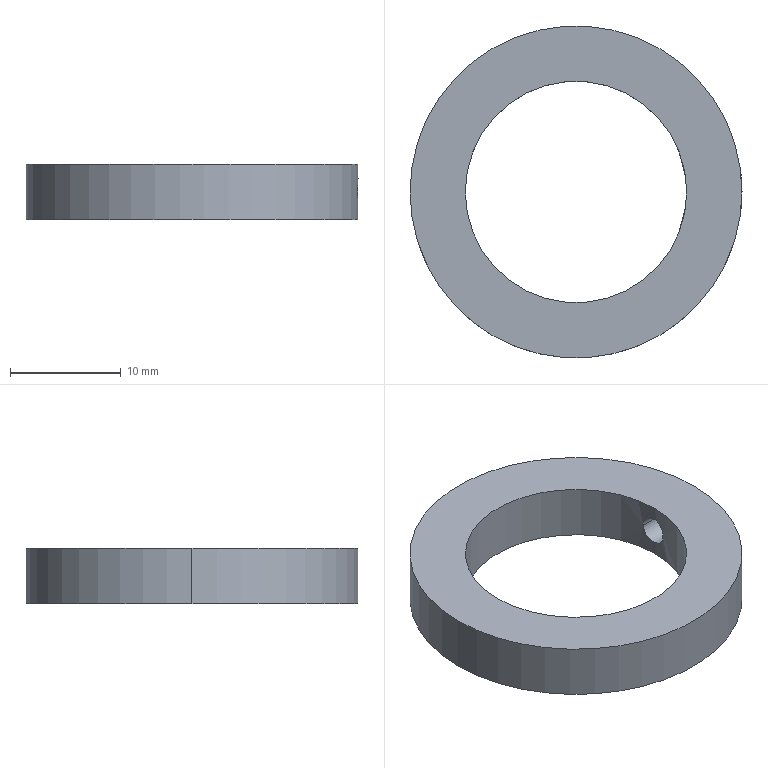Part | SolidWorks | features 3DProfileFeature 1, Extrusion 1, HoleWzd 1 | 1 solid | 8 faces | box 30 x 30 x 5 mm | volume 1939 mm3 | cylinder 6 | plane 2 | commonest cylinder face diameters 2.5 x2 20 x2 30 x2
STEP:
#1=CARTESIAN_POINT('',(10.,0.,1.252));
#2=VERTEX_POINT('',#1);
#3=CARTESIAN_POINT('',(9.93,-1.183,2.5));
#4=VERTEX_POINT('',#3);
#5=CARTESIAN_POINT('',(10.,0.,1.252));
#6=CARTESIAN_POINT('',(10.,-0.1581,1.26));
#7=CARTESIAN_POINT('',(9.996,-0.3132,1.299));
#8=CARTESIAN_POINT('',(9.983,-0.602,1.433));
#9=CARTESIAN_POINT('',(9.974,-0.7312,1.525));
#10=CARTESIAN_POINT('',(9.955,-0.9493,1.756));
#11=CARTESIAN_POINT('',(9.946,-1.035,1.891));
#12=CARTESIAN_POINT('',(9.934,-1.152,2.184));
#13=CARTESIAN_POINT('',(9.93,-1.183,2.342));
#14=CARTESIAN_POINT('',(9.93,-1.183,2.5));
#15=B_SPLINE_CURVE_WITH_KNOTS('',3,(#5,#6,#7,#8,#9,#10,#11,#12,#13,#14),.UNSPECIFIED.,.F.,.F.,(4,2,2,2,4),(0.002024,0.002496,0.002968,0.00344,0.003912),.UNSPECIFIED.);
#16=EDGE_CURVE('',#2,#4,#15,.T.);
#17=ORIENTED_EDGE('',*,*,#16,.T.);
#18=CARTESIAN_POINT('',(14.956,-1.149,2.5));
#19=VERTEX_POINT('',#18);
#20=CARTESIAN_POINT('',(15.008,-1.148,2.5));
#21=DIRECTION('',(1.,0.00677,0.));
#22=VECTOR('',#21,1000.);
#23=LINE('',#20,#22);
#24=EDGE_CURVE('',#4,#19,#23,.T.);
#25=ORIENTED_EDGE('',*,*,#24,.T.);
#26=CARTESIAN_POINT('',(15.,0.,1.254));
#27=VERTEX_POINT('',#26);
#28=CARTESIAN_POINT('',(15.,0.,1.254));
#29=CARTESIAN_POINT('',(15.,-0.3107,1.279));
#30=CARTESIAN_POINT('',(14.989,-0.6069,1.424));
#31=CARTESIAN_POINT('',(14.972,-0.9234,1.767));
#32=CARTESIAN_POINT('',(14.966,-1.007,1.901));
#33=CARTESIAN_POINT('',(14.958,-1.12,2.19));
#34=CARTESIAN_POINT('',(14.956,-1.149,2.345));
#35=CARTESIAN_POINT('',(14.956,-1.149,2.5));
#36=B_SPLINE_CURVE_WITH_KNOTS('',3,(#28,#29,#30,#31,#32,#33,#34,#35),.UNSPECIFIED.,.F.,.F.,(4,2,2,4),(0.002057,0.002983,0.003446,0.00391),.UNSPECIFIED.);
#37=EDGE_CURVE('',#27,#19,#36,.T.);
#38=ORIENTED_EDGE('',*,*,#37,.F.);
#39=CARTESIAN_POINT('',(14.939,1.351,2.5));
#40=VERTEX_POINT('',#39);
#41=CARTESIAN_POINT('',(14.939,1.351,2.5));
#42=CARTESIAN_POINT('',(14.939,1.351,2.413));
#43=CARTESIAN_POINT('',(14.94,1.342,2.328));
#44=CARTESIAN_POINT('',(14.943,1.307,2.16));
#45=CARTESIAN_POINT('',(14.945,1.28,2.076));
#46=CARTESIAN_POINT('',(14.954,1.177,1.84));
#47=CARTESIAN_POINT('',(14.962,1.074,1.697));
#48=CARTESIAN_POINT('',(14.978,0.8225,1.465));
#49=CARTESIAN_POINT('',(14.986,0.671,1.374));
#50=CARTESIAN_POINT('',(14.994,0.4277,1.29));
#51=CARTESIAN_POINT('',(14.996,0.3423,1.27));
#52=CARTESIAN_POINT('',(14.999,0.1719,1.249));
#53=CARTESIAN_POINT('',(15.,0.0862,1.247));
#54=CARTESIAN_POINT('',(15.,0.,1.254));
#55=B_SPLINE_CURVE_WITH_KNOTS('',3,(#41,#42,#43,#44,#45,#46,#47,#48,#49,#50,#51,#52,#53,#54),.UNSPECIFIED.,.F.,.F.,(4,2,2,2,2,2,4),(0.,0.0002571,0.0005141,0.001028,0.001542,0.001799,0.002057),.UNSPECIFIED.);
#56=EDGE_CURVE('',#40,#27,#55,.T.);
#57=ORIENTED_EDGE('',*,*,#56,.F.);
#58=CARTESIAN_POINT('',(9.913,1.317,2.5));
#59=VERTEX_POINT('',#58);
#60=CARTESIAN_POINT('',(14.991,1.352,2.5));
#61=DIRECTION('',(1.,0.00677,0.));
#62=VECTOR('',#61,1000.);
#63=LINE('',#60,#62);
#64=EDGE_CURVE('',#59,#40,#63,.T.);
#65=ORIENTED_EDGE('',*,*,#64,.F.);
#66=CARTESIAN_POINT('',(9.913,1.317,2.5));
#67=CARTESIAN_POINT('',(9.913,1.317,2.414));
#68=CARTESIAN_POINT('',(9.914,1.308,2.33));
#69=CARTESIAN_POINT('',(9.918,1.274,2.165));
#70=CARTESIAN_POINT('',(9.922,1.249,2.083));
#71=CARTESIAN_POINT('',(9.934,1.148,1.85));
#72=CARTESIAN_POINT('',(9.946,1.049,1.708));
#73=CARTESIAN_POINT('',(9.968,0.8046,1.476));
#74=CARTESIAN_POINT('',(9.98,0.6572,1.385));
#75=CARTESIAN_POINT('',(9.991,0.4198,1.298));
#76=CARTESIAN_POINT('',(9.995,0.3364,1.276));
#77=CARTESIAN_POINT('',(9.999,0.1689,1.251));
#78=CARTESIAN_POINT('',(10.,0.08472,1.247));
#79=CARTESIAN_POINT('',(10.,0.,1.252));
#80=B_SPLINE_CURVE_WITH_KNOTS('',3,(#66,#67,#68,#69,#70,#71,#72,#73,#74,#75,#76,#77,#78,#79),.UNSPECIFIED.,.F.,.F.,(4,2,2,2,2,2,4),(0.,0.000253,0.000506,0.001012,0.001518,0.001771,0.002024),.UNSPECIFIED.);
#81=EDGE_CURVE('',#59,#2,#80,.T.);
#82=ORIENTED_EDGE('',*,*,#81,.T.);
#83=EDGE_LOOP('',(#17,#25,#38,#57,#65,#82));
#84=FACE_OUTER_BOUND('',#83,.T.);
#85=CARTESIAN_POINT('',(15.,0.1016,2.5));
#86=DIRECTION('',(1.,0.00677,0.));
#87=DIRECTION('',(-0.00677,1.,0.));
#88=AXIS2_PLACEMENT_3D('',#85,#86,#87);
#89=CYLINDRICAL_SURFACE('',#88,1.25);
#90=ADVANCED_FACE('',(#84),#89,.F.);
#91=CARTESIAN_POINT('',(-10.,0.,5.));
#92=VERTEX_POINT('',#91);
#93=CARTESIAN_POINT('',(10.,0.,5.));
#94=VERTEX_POINT('',#93);
#95=CARTESIAN_POINT('',(0.,0.,5.));
#96=DIRECTION('',(0.,0.,1.));
#97=DIRECTION('',(1.,0.,0.));
#98=AXIS2_PLACEMENT_3D('',#95,#96,#97);
#99=CIRCLE('',#98,10.);
#100=EDGE_CURVE('',#92,#94,#99,.T.);
#101=ORIENTED_EDGE('',*,*,#100,.T.);
#102=CARTESIAN_POINT('',(10.,0.,3.748));
#103=VERTEX_POINT('',#102);
#104=CARTESIAN_POINT('',(10.,0.,5.));
#105=DIRECTION('',(0.,0.,-1.));
#106=VECTOR('',#105,1000.);
#107=LINE('',#104,#106);
#108=EDGE_CURVE('',#94,#103,#107,.T.);
#109=ORIENTED_EDGE('',*,*,#108,.T.);
#110=CARTESIAN_POINT('',(9.93,-1.183,2.5));
#111=CARTESIAN_POINT('',(9.93,-1.183,2.658));
#112=CARTESIAN_POINT('',(9.934,-1.152,2.817));
#113=CARTESIAN_POINT('',(9.946,-1.036,3.109));
#114=CARTESIAN_POINT('',(9.956,-0.9483,3.245));
#115=CARTESIAN_POINT('',(9.974,-0.7319,3.474));
#116=CARTESIAN_POINT('',(9.983,-0.6007,3.568));
#117=CARTESIAN_POINT('',(9.996,-0.3145,3.701));
#118=CARTESIAN_POINT('',(10.,-0.1583,3.74));
#119=CARTESIAN_POINT('',(10.,0.,3.748));
#120=B_SPLINE_CURVE_WITH_KNOTS('',3,(#110,#111,#112,#113,#114,#115,#116,#117,#118,#119),.UNSPECIFIED.,.F.,.F.,(4,2,2,2,4),(0.003912,0.004384,0.004857,0.005329,0.005801),.UNSPECIFIED.);
#121=EDGE_CURVE('',#4,#103,#120,.T.);
#122=ORIENTED_EDGE('',*,*,#121,.F.);
#123=ORIENTED_EDGE('',*,*,#16,.F.);
#124=CARTESIAN_POINT('',(10.,0.,0.));
#125=VERTEX_POINT('',#124);
#126=CARTESIAN_POINT('',(10.,0.,5.));
#127=DIRECTION('',(0.,0.,-1.));
#128=VECTOR('',#127,1000.);
#129=LINE('',#126,#128);
#130=EDGE_CURVE('',#2,#125,#129,.T.);
#131=ORIENTED_EDGE('',*,*,#130,.T.);
#132=CARTESIAN_POINT('',(-10.,0.,0.));
#133=VERTEX_POINT('',#132);
#134=CARTESIAN_POINT('',(0.,0.,0.));
#135=DIRECTION('',(0.,0.,1.));
#136=DIRECTION('',(1.,0.,0.));
#137=AXIS2_PLACEMENT_3D('',#134,#135,#136);
#138=CIRCLE('',#137,10.);
#139=EDGE_CURVE('',#133,#125,#138,.T.);
#140=ORIENTED_EDGE('',*,*,#139,.F.);
#141=CARTESIAN_POINT('',(-10.,0.,5.));
#142=DIRECTION('',(0.,0.,-1.));
#143=VECTOR('',#142,1000.);
#144=LINE('',#141,#143);
#145=EDGE_CURVE('',#92,#133,#144,.T.);
#146=ORIENTED_EDGE('',*,*,#145,.F.);
#147=EDGE_LOOP('',(#101,#109,#122,#123,#131,#140,#146));
#148=FACE_OUTER_BOUND('',#147,.T.);
#149=CARTESIAN_POINT('',(0.,0.,5.));
#150=DIRECTION('',(0.,0.,-1.));
#151=DIRECTION('',(-1.,0.,0.));
#152=AXIS2_PLACEMENT_3D('',#149,#150,#151);
#153=CYLINDRICAL_SURFACE('',#152,10.);
#154=ADVANCED_FACE('',(#148),#153,.F.);
#155=CARTESIAN_POINT('',(15.,0.,5.));
#156=VERTEX_POINT('',#155);
#157=CARTESIAN_POINT('',(-15.,0.,5.));
#158=VERTEX_POINT('',#157);
#159=CARTESIAN_POINT('',(0.,0.,5.));
#160=DIRECTION('',(0.,0.,1.));
#161=DIRECTION('',(1.,0.,0.));
#162=AXIS2_PLACEMENT_3D('',#159,#160,#161);
#163=CIRCLE('',#162,15.);
#164=EDGE_CURVE('',#156,#158,#163,.T.);
#165=ORIENTED_EDGE('',*,*,#164,.F.);
#166=CARTESIAN_POINT('',(15.,0.,3.746));
#167=VERTEX_POINT('',#166);
#168=CARTESIAN_POINT('',(15.,0.,5.));
#169=DIRECTION('',(0.,0.,-1.));
#170=VECTOR('',#169,1000.);
#171=LINE('',#168,#170);
#172=EDGE_CURVE('',#156,#167,#171,.T.);
#173=ORIENTED_EDGE('',*,*,#172,.T.);
#174=CARTESIAN_POINT('',(15.,0.,3.746));
#175=CARTESIAN_POINT('',(15.,0.0856,3.753));
#176=CARTESIAN_POINT('',(14.999,0.1731,3.751));
#177=CARTESIAN_POINT('',(14.996,0.3431,3.729));
#178=CARTESIAN_POINT('',(14.994,0.4266,3.71));
#179=CARTESIAN_POINT('',(14.986,0.6724,3.625));
#180=CARTESIAN_POINT('',(14.978,0.8221,3.536));
#181=CARTESIAN_POINT('',(14.962,1.075,3.303));
#182=CARTESIAN_POINT('',(14.954,1.177,3.159));
#183=CARTESIAN_POINT('',(14.942,1.315,2.846));
#184=CARTESIAN_POINT('',(14.939,1.351,2.674));
#185=CARTESIAN_POINT('',(14.939,1.351,2.5));
#186=B_SPLINE_CURVE_WITH_KNOTS('',3,(#174,#175,#176,#177,#178,#179,#180,#181,#182,#183,#184,#185),.UNSPECIFIED.,.F.,.F.,(4,2,2,2,2,4),(0.005764,0.006021,0.006278,0.006791,0.007305,0.007819),.UNSPECIFIED.);
#187=EDGE_CURVE('',#167,#40,#186,.T.);
#188=ORIENTED_EDGE('',*,*,#187,.T.);
#189=ORIENTED_EDGE('',*,*,#56,.T.);
#190=CARTESIAN_POINT('',(15.,0.,0.));
#191=VERTEX_POINT('',#190);
#192=CARTESIAN_POINT('',(15.,0.,5.));
#193=DIRECTION('',(0.,0.,-1.));
#194=VECTOR('',#193,1000.);
#195=LINE('',#192,#194);
#196=EDGE_CURVE('',#27,#191,#195,.T.);
#197=ORIENTED_EDGE('',*,*,#196,.T.);
#198=CARTESIAN_POINT('',(-15.,0.,0.));
#199=VERTEX_POINT('',#198);
#200=CARTESIAN_POINT('',(0.,0.,0.));
#201=DIRECTION('',(0.,0.,1.));
#202=DIRECTION('',(1.,0.,0.));
#203=AXIS2_PLACEMENT_3D('',#200,#201,#202);
#204=CIRCLE('',#203,15.);
#205=EDGE_CURVE('',#191,#199,#204,.T.);
#206=ORIENTED_EDGE('',*,*,#205,.T.);
#207=CARTESIAN_POINT('',(-15.,0.,5.));
#208=DIRECTION('',(0.,0.,-1.));
#209=VECTOR('',#208,1000.);
#210=LINE('',#207,#209);
#211=EDGE_CURVE('',#158,#199,#210,.T.);
#212=ORIENTED_EDGE('',*,*,#211,.F.);
#213=EDGE_LOOP('',(#165,#173,#188,#189,#197,#206,#212));
#214=FACE_OUTER_BOUND('',#213,.T.);
#215=CARTESIAN_POINT('',(0.,0.,5.));
#216=DIRECTION('',(0.,0.,-1.));
#217=DIRECTION('',(-1.,0.,0.));
#218=AXIS2_PLACEMENT_3D('',#215,#216,#217);
#219=CYLINDRICAL_SURFACE('',#218,15.);
#220=ADVANCED_FACE('',(#214),#219,.T.);
#221=CARTESIAN_POINT('',(0.,0.,5.));
#222=DIRECTION('',(0.,0.,1.));
#223=DIRECTION('',(1.,0.,0.));
#224=AXIS2_PLACEMENT_3D('',#221,#222,#223);
#225=CIRCLE('',#224,15.);
#226=EDGE_CURVE('',#158,#156,#225,.T.);
#227=ORIENTED_EDGE('',*,*,#226,.T.);
#228=ORIENTED_EDGE('',*,*,#164,.T.);
#229=EDGE_LOOP('',(#227,#228));
#230=FACE_OUTER_BOUND('',#229,.T.);
#231=ORIENTED_EDGE('',*,*,#100,.F.);
#232=CARTESIAN_POINT('',(0.,0.,5.));
#233=DIRECTION('',(0.,0.,1.));
#234=DIRECTION('',(1.,0.,0.));
#235=AXIS2_PLACEMENT_3D('',#232,#233,#234);
#236=CIRCLE('',#235,10.);
#237=EDGE_CURVE('',#94,#92,#236,.T.);
#238=ORIENTED_EDGE('',*,*,#237,.F.);
#239=EDGE_LOOP('',(#231,#238));
#240=FACE_BOUND('',#239,.T.);
#241=CARTESIAN_POINT('',(0.,0.,5.));
#242=DIRECTION('',(0.,0.,1.));
#243=DIRECTION('',(1.,0.,0.));
#244=AXIS2_PLACEMENT_3D('',#241,#242,#243);
#245=PLANE('',#244);
#246=ADVANCED_FACE('',(#230,#240),#245,.T.);
#247=CARTESIAN_POINT('',(0.,0.,0.));
#248=DIRECTION('',(0.,0.,1.));
#249=DIRECTION('',(1.,0.,0.));
#250=AXIS2_PLACEMENT_3D('',#247,#248,#249);
#251=CIRCLE('',#250,15.);
#252=EDGE_CURVE('',#199,#191,#251,.T.);
#253=ORIENTED_EDGE('',*,*,#252,.F.);
#254=ORIENTED_EDGE('',*,*,#205,.F.);
#255=EDGE_LOOP('',(#253,#254));
#256=FACE_OUTER_BOUND('',#255,.T.);
#257=ORIENTED_EDGE('',*,*,#139,.T.);
#258=CARTESIAN_POINT('',(0.,0.,0.));
#259=DIRECTION('',(0.,0.,1.));
#260=DIRECTION('',(1.,0.,0.));
#261=AXIS2_PLACEMENT_3D('',#258,#259,#260);
#262=CIRCLE('',#261,10.);
#263=EDGE_CURVE('',#125,#133,#262,.T.);
#264=ORIENTED_EDGE('',*,*,#263,.T.);
#265=EDGE_LOOP('',(#257,#264));
#266=FACE_BOUND('',#265,.T.);
#267=CARTESIAN_POINT('',(0.,0.,0.));
#268=DIRECTION('',(0.,0.,1.));
#269=DIRECTION('',(1.,0.,0.));
#270=AXIS2_PLACEMENT_3D('',#267,#268,#269);
#271=PLANE('',#270);
#272=ADVANCED_FACE('',(#256,#266),#271,.F.);
#273=ORIENTED_EDGE('',*,*,#172,.F.);
#274=ORIENTED_EDGE('',*,*,#226,.F.);
#275=ORIENTED_EDGE('',*,*,#211,.T.);
#276=ORIENTED_EDGE('',*,*,#252,.T.);
#277=ORIENTED_EDGE('',*,*,#196,.F.);
#278=ORIENTED_EDGE('',*,*,#37,.T.);
#279=CARTESIAN_POINT('',(14.956,-1.149,2.5));
#280=CARTESIAN_POINT('',(14.956,-1.149,2.655));
#281=CARTESIAN_POINT('',(14.958,-1.119,2.811));
#282=CARTESIAN_POINT('',(14.966,-1.007,3.099));
#283=CARTESIAN_POINT('',(14.972,-0.9224,3.234));
#284=CARTESIAN_POINT('',(14.983,-0.713,3.461));
#285=CARTESIAN_POINT('',(14.989,-0.5855,3.556));
#286=CARTESIAN_POINT('',(14.997,-0.3075,3.691));
#287=CARTESIAN_POINT('',(15.,-0.1545,3.733));
#288=CARTESIAN_POINT('',(15.,0.,3.746));
#289=B_SPLINE_CURVE_WITH_KNOTS('',3,(#279,#280,#281,#282,#283,#284,#285,#286,#287,#288),.UNSPECIFIED.,.F.,.F.,(4,2,2,2,4),(0.00391,0.004373,0.004837,0.005301,0.005764),.UNSPECIFIED.);
#290=EDGE_CURVE('',#19,#167,#289,.T.);
#291=ORIENTED_EDGE('',*,*,#290,.T.);
#292=EDGE_LOOP('',(#273,#274,#275,#276,#277,#278,#291));
#293=FACE_OUTER_BOUND('',#292,.T.);
#294=CARTESIAN_POINT('',(0.,0.,5.));
#295=DIRECTION('',(0.,0.,-1.));
#296=DIRECTION('',(-1.,0.,0.));
#297=AXIS2_PLACEMENT_3D('',#294,#295,#296);
#298=CYLINDRICAL_SURFACE('',#297,15.);
#299=ADVANCED_FACE('',(#293),#298,.T.);
#300=ORIENTED_EDGE('',*,*,#108,.F.);
#301=ORIENTED_EDGE('',*,*,#237,.T.);
#302=ORIENTED_EDGE('',*,*,#145,.T.);
#303=ORIENTED_EDGE('',*,*,#263,.F.);
#304=ORIENTED_EDGE('',*,*,#130,.F.);
#305=ORIENTED_EDGE('',*,*,#81,.F.);
#306=CARTESIAN_POINT('',(10.,0.,3.748));
#307=CARTESIAN_POINT('',(10.,0.1694,3.757));
#308=CARTESIAN_POINT('',(9.996,0.3394,3.732));
#309=CARTESIAN_POINT('',(9.984,0.579,3.644));
#310=CARTESIAN_POINT('',(9.979,0.6546,3.607));
#311=CARTESIAN_POINT('',(9.968,0.7977,3.518));
#312=CARTESIAN_POINT('',(9.963,0.8658,3.466));
#313=CARTESIAN_POINT('',(9.946,1.049,3.292));
#314=CARTESIAN_POINT('',(9.934,1.148,3.15));
#315=CARTESIAN_POINT('',(9.918,1.282,2.841));
#316=CARTESIAN_POINT('',(9.913,1.317,2.671));
#317=CARTESIAN_POINT('',(9.913,1.317,2.5));
#318=B_SPLINE_CURVE_WITH_KNOTS('',3,(#306,#307,#308,#309,#310,#311,#312,#313,#314,#315,#316,#317),.UNSPECIFIED.,.F.,.F.,(4,2,2,2,2,4),(0.005801,0.006307,0.006559,0.006812,0.007317,0.007823),.UNSPECIFIED.);
#319=EDGE_CURVE('',#103,#59,#318,.T.);
#320=ORIENTED_EDGE('',*,*,#319,.F.);
#321=EDGE_LOOP('',(#300,#301,#302,#303,#304,#305,#320));
#322=FACE_OUTER_BOUND('',#321,.T.);
#323=CARTESIAN_POINT('',(0.,0.,5.));
#324=DIRECTION('',(0.,0.,-1.));
#325=DIRECTION('',(-1.,0.,0.));
#326=AXIS2_PLACEMENT_3D('',#323,#324,#325);
#327=CYLINDRICAL_SURFACE('',#326,10.);
#328=ADVANCED_FACE('',(#322),#327,.F.);
#329=ORIENTED_EDGE('',*,*,#24,.F.);
#330=ORIENTED_EDGE('',*,*,#121,.T.);
#331=ORIENTED_EDGE('',*,*,#319,.T.);
#332=ORIENTED_EDGE('',*,*,#64,.T.);
#333=ORIENTED_EDGE('',*,*,#187,.F.);
#334=ORIENTED_EDGE('',*,*,#290,.F.);
#335=EDGE_LOOP('',(#329,#330,#331,#332,#333,#334));
#336=FACE_OUTER_BOUND('',#335,.T.);
#337=CARTESIAN_POINT('',(15.,0.1016,2.5));
#338=DIRECTION('',(1.,0.00677,0.));
#339=DIRECTION('',(-0.00677,1.,0.));
#340=AXIS2_PLACEMENT_3D('',#337,#338,#339);
#341=CYLINDRICAL_SURFACE('',#340,1.25);
#342=ADVANCED_FACE('',(#336),#341,.F.);
#343=CLOSED_SHELL('',(#90,#154,#220,#246,#272,#299,#328,#342));
#344=MANIFOLD_SOLID_BREP('',#343);
#345=CARTESIAN_POINT('',(0.,0.,0.));
#346=DIRECTION('',(0.,0.,1.));
#347=DIRECTION('',(1.,0.,0.));
#348=AXIS2_PLACEMENT_3D('',#345,#346,#347);
#349=(LENGTH_UNIT()NAMED_UNIT(*)SI_UNIT(.MILLI.,.METRE.));
#350=UNCERTAINTY_MEASURE_WITH_UNIT(LENGTH_MEASURE(0.00001),#349,'','');
#351=(NAMED_UNIT(*)PLANE_ANGLE_UNIT()SI_UNIT($,.RADIAN.));
#352=(NAMED_UNIT(*)SI_UNIT($,.STERADIAN.)SOLID_ANGLE_UNIT());
#353=(GEOMETRIC_REPRESENTATION_CONTEXT(3)GLOBAL_UNCERTAINTY_ASSIGNED_CONTEXT((#350))GLOBAL_UNIT_ASSIGNED_CONTEXT((#349,#351,#352))REPRESENTATION_CONTEXT('',''));
#354=ADVANCED_BREP_SHAPE_REPRESENTATION('',(#344,#348),#353);